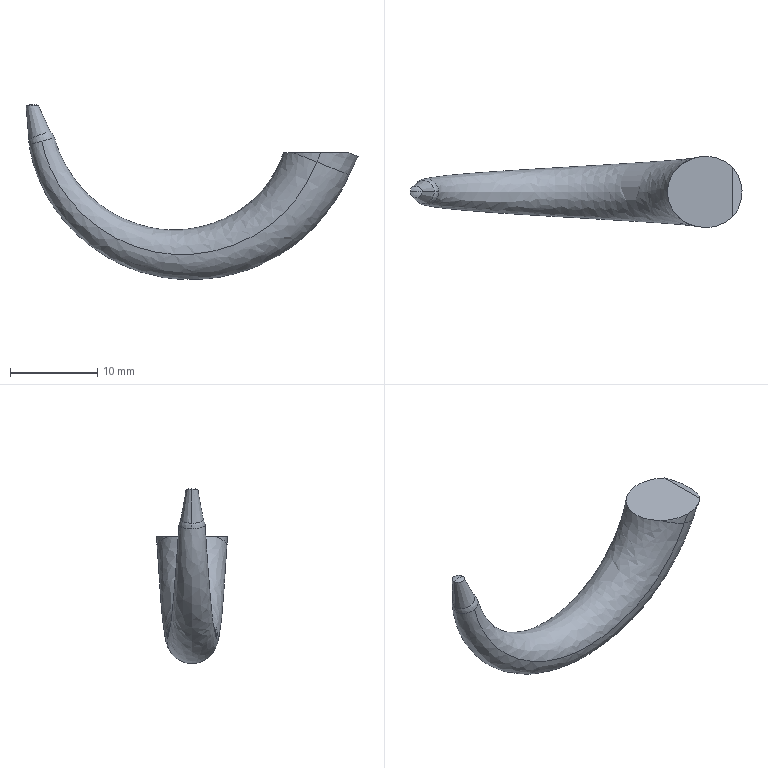Part | Creo | 1 solid | 13 faces | box 38.084 x 8.15 x 20.091 mm | volume 1170 mm3 | spline 5 | sphere 4 | plane 2 | cone 2
STEP:
#1=CARTESIAN_POINT('',(-144.079,122.31,36.852));
#2=VERTEX_POINT('',#1);
#3=CARTESIAN_POINT('',(-144.079,127.996,36.852));
#4=VERTEX_POINT('',#3);
#5=CARTESIAN_POINT('',(-144.079,122.31,36.852));
#6=DIRECTION('',(-0.000000028,1.,-0.000000063));
#7=VECTOR('',#6,5.687);
#8=LINE('',#5,#7);
#9=EDGE_CURVE('',#2,#4,#8,.T.);
#10=ORIENTED_EDGE('',*,*,#9,.F.);
#11=CARTESIAN_POINT('',(-147.308,121.079,36.852));
#12=VERTEX_POINT('',#11);
#13=CARTESIAN_POINT('',(-144.079,122.31,36.852));
#14=CARTESIAN_POINT('',(-144.243,122.153,36.852));
#15=CARTESIAN_POINT('',(-144.595,121.866,36.852));
#16=CARTESIAN_POINT('',(-145.204,121.513,36.852));
#17=CARTESIAN_POINT('',(-145.872,121.255,36.852));
#18=CARTESIAN_POINT('',(-146.584,121.102,36.852));
#19=CARTESIAN_POINT('',(-147.064,121.074,36.852));
#20=CARTESIAN_POINT('',(-147.308,121.079,36.852));
#21=B_SPLINE_CURVE_WITH_KNOTS('',3,(#13,#14,#15,#16,#17,#18,#19,#20),.UNSPECIFIED.,.F.,.F.,(4,1,1,1,1,4),(0.,0.2,0.4,0.6,0.8,1.),.UNSPECIFIED.);
#22=EDGE_CURVE('',#2,#12,#21,.T.);
#23=ORIENTED_EDGE('',*,*,#22,.T.);
#24=CARTESIAN_POINT('',(-150.452,122.415,36.852));
#25=VERTEX_POINT('',#24);
#26=CARTESIAN_POINT('',(-147.308,121.079,36.852));
#27=CARTESIAN_POINT('',(-147.55,121.084,36.852));
#28=CARTESIAN_POINT('',(-148.025,121.13,36.852));
#29=CARTESIAN_POINT('',(-148.724,121.309,36.852));
#30=CARTESIAN_POINT('',(-149.372,121.588,36.852));
#31=CARTESIAN_POINT('',(-149.957,121.957,36.852));
#32=CARTESIAN_POINT('',(-150.296,122.254,36.852));
#33=CARTESIAN_POINT('',(-150.451,122.414,36.852));
#34=B_SPLINE_CURVE_WITH_KNOTS('',3,(#26,#27,#28,#29,#30,#31,#32,#33),.UNSPECIFIED.,.F.,.F.,(4,1,1,1,1,4),(0.,0.2,0.4,0.6,0.8,1.),.UNSPECIFIED.);
#35=EDGE_CURVE('',#12,#25,#34,.T.);
#36=ORIENTED_EDGE('',*,*,#35,.T.);
#37=CARTESIAN_POINT('',(-150.452,127.891,36.852));
#38=VERTEX_POINT('',#37);
#39=CARTESIAN_POINT('',(-150.451,122.414,36.852));
#40=CARTESIAN_POINT('',(-150.618,122.585,36.852));
#41=CARTESIAN_POINT('',(-150.912,122.943,36.852));
#42=CARTESIAN_POINT('',(-151.252,123.538,36.852));
#43=CARTESIAN_POINT('',(-151.48,124.169,36.852));
#44=CARTESIAN_POINT('',(-151.596,124.824,36.852));
#45=CARTESIAN_POINT('',(-151.596,125.483,36.852));
#46=CARTESIAN_POINT('',(-151.48,126.137,36.852));
#47=CARTESIAN_POINT('',(-151.251,126.77,36.852));
#48=CARTESIAN_POINT('',(-150.91,127.364,36.852));
#49=CARTESIAN_POINT('',(-150.617,127.721,36.852));
#50=CARTESIAN_POINT('',(-150.452,127.892,36.852));
#51=B_SPLINE_CURVE_WITH_KNOTS('',3,(#39,#40,#41,#42,#43,#44,#45,#46,#47,#48,#49,#50),.UNSPECIFIED.,.F.,.F.,(4,1,1,1,1,1,1,1,1,4),(0.,0.1111,0.2222,0.3333,0.4444,0.5556,0.6667,0.7778,0.8889,1.),.UNSPECIFIED.);
#52=EDGE_CURVE('',#25,#38,#51,.T.);
#53=ORIENTED_EDGE('',*,*,#52,.T.);
#54=CARTESIAN_POINT('',(-147.308,129.227,36.852));
#55=VERTEX_POINT('',#54);
#56=CARTESIAN_POINT('',(-150.452,127.892,36.852));
#57=CARTESIAN_POINT('',(-150.296,128.052,36.852));
#58=CARTESIAN_POINT('',(-149.958,128.349,36.852));
#59=CARTESIAN_POINT('',(-149.373,128.717,36.852));
#60=CARTESIAN_POINT('',(-148.725,128.997,36.852));
#61=CARTESIAN_POINT('',(-148.029,129.175,36.852));
#62=CARTESIAN_POINT('',(-147.551,129.222,36.852));
#63=CARTESIAN_POINT('',(-147.308,129.227,36.852));
#64=B_SPLINE_CURVE_WITH_KNOTS('',3,(#56,#57,#58,#59,#60,#61,#62,#63),.UNSPECIFIED.,.F.,.F.,(4,1,1,1,1,4),(0.,0.2,0.4,0.6,0.8,1.),.UNSPECIFIED.);
#65=EDGE_CURVE('',#38,#55,#64,.T.);
#66=ORIENTED_EDGE('',*,*,#65,.T.);
#67=CARTESIAN_POINT('',(-144.079,127.996,36.852));
#68=CARTESIAN_POINT('',(-144.216,128.127,36.852));
#69=CARTESIAN_POINT('',(-144.506,128.369,36.852));
#70=CARTESIAN_POINT('',(-144.996,128.68,36.852));
#71=CARTESIAN_POINT('',(-145.532,128.928,36.852));
#72=CARTESIAN_POINT('',(-146.104,129.108,36.852));
#73=CARTESIAN_POINT('',(-146.7,129.213,36.852));
#74=CARTESIAN_POINT('',(-147.104,129.231,36.852));
#75=CARTESIAN_POINT('',(-147.308,129.227,36.852));
#76=B_SPLINE_CURVE_WITH_KNOTS('',3,(#67,#68,#69,#70,#71,#72,#73,#74,#75),.UNSPECIFIED.,.F.,.F.,(4,1,1,1,1,1,4),(0.,0.1667,0.3333,0.5,0.6667,0.8333,1.),.UNSPECIFIED.);
#77=EDGE_CURVE('',#4,#55,#76,.T.);
#78=ORIENTED_EDGE('',*,*,#77,.F.);
#79=EDGE_LOOP('',(#10,#23,#36,#53,#66,#78));
#80=FACE_OUTER_BOUND('',#79,.F.);
#81=CARTESIAN_POINT('',(-151.801,125.153,36.852));
#82=DIRECTION('',(0.,0.,1.));
#83=DIRECTION('',(1.,0.,0.));
#84=AXIS2_PLACEMENT_3D('',#81,#82,#83);
#85=PLANE('',#84);
#86=ADVANCED_FACE('',(#80),#85,.T.);
#87=CARTESIAN_POINT('',(-144.079,127.996,36.852));
#88=CARTESIAN_POINT('',(-143.93,127.825,36.793));
#89=CARTESIAN_POINT('',(-143.662,127.463,36.687));
#90=CARTESIAN_POINT('',(-143.348,126.85,36.562));
#91=CARTESIAN_POINT('',(-143.134,126.191,36.477));
#92=CARTESIAN_POINT('',(-143.026,125.502,36.434));
#93=CARTESIAN_POINT('',(-143.026,124.804,36.434));
#94=CARTESIAN_POINT('',(-143.134,124.115,36.477));
#95=CARTESIAN_POINT('',(-143.348,123.456,36.562));
#96=CARTESIAN_POINT('',(-143.662,122.843,36.687));
#97=CARTESIAN_POINT('',(-143.93,122.481,36.793));
#98=CARTESIAN_POINT('',(-144.079,122.31,36.852));
#99=B_SPLINE_CURVE_WITH_KNOTS('',3,(#87,#88,#89,#90,#91,#92,#93,#94,#95,#96,#97,#98),.UNSPECIFIED.,.F.,.F.,(4,1,1,1,1,1,1,1,1,4),(0.,0.1111,0.2222,0.3333,0.4444,0.5556,0.6667,0.7778,0.8889,1.),.UNSPECIFIED.);
#100=EDGE_CURVE('',#4,#2,#99,.T.);
#101=ORIENTED_EDGE('',*,*,#100,.T.);
#102=ORIENTED_EDGE('',*,*,#9,.T.);
#103=EDGE_LOOP('',(#101,#102));
#104=FACE_OUTER_BOUND('',#103,.F.);
#105=CARTESIAN_POINT('',(-145.561,129.153,37.44));
#106=DIRECTION('',(0.3687,0.,0.9295));
#107=DIRECTION('',(-0.9295,0.,0.3687));
#108=AXIS2_PLACEMENT_3D('',#105,#106,#107);
#109=PLANE('',#108);
#110=ADVANCED_FACE('',(#104),#109,.T.);
#111=ORIENTED_EDGE('',*,*,#22,.F.);
#112=ORIENTED_EDGE('',*,*,#100,.F.);
#113=ORIENTED_EDGE('',*,*,#77,.T.);
#114=CARTESIAN_POINT('',(-147.742,129.153,35.777));
#115=VERTEX_POINT('',#114);
#116=CARTESIAN_POINT('',(-147.308,129.227,36.852));
#117=DIRECTION('',(-0.3736,-0.06365,-0.9254));
#118=VECTOR('',#117,1.162);
#119=LINE('',#116,#118);
#120=EDGE_CURVE('',#55,#115,#119,.T.);
#121=ORIENTED_EDGE('',*,*,#120,.T.);
#122=CARTESIAN_POINT('',(-147.742,121.153,35.777));
#123=VERTEX_POINT('',#122);
#124=CARTESIAN_POINT('',(-147.742,125.153,35.777));
#125=DIRECTION('',(0.3687,0.,0.9295));
#126=DIRECTION('',(0.,-1.,0.));
#127=AXIS2_PLACEMENT_3D('',#124,#125,#126);
#128=CIRCLE('',#127,4.);
#129=EDGE_CURVE('',#123,#115,#128,.T.);
#130=ORIENTED_EDGE('',*,*,#129,.F.);
#131=CARTESIAN_POINT('',(-147.308,121.079,36.852));
#132=DIRECTION('',(-0.3735,0.06365,-0.9254));
#133=VECTOR('',#132,1.162);
#134=LINE('',#131,#133);
#135=EDGE_CURVE('',#12,#123,#134,.T.);
#136=ORIENTED_EDGE('',*,*,#135,.F.);
#137=EDGE_LOOP('',(#111,#112,#113,#121,#130,#136));
#138=FACE_OUTER_BOUND('',#137,.F.);
#139=CARTESIAN_POINT('',(-147.195,121.027,37.769));
#140=CARTESIAN_POINT('',(-147.462,121.073,37.12));
#141=CARTESIAN_POINT('',(-147.728,121.119,36.471));
#142=CARTESIAN_POINT('',(-147.995,121.164,35.821));
#143=CARTESIAN_POINT('',(-147.117,121.023,37.748));
#144=CARTESIAN_POINT('',(-147.384,121.068,37.095));
#145=CARTESIAN_POINT('',(-147.651,121.114,36.443));
#146=CARTESIAN_POINT('',(-147.918,121.159,35.79));
#147=CARTESIAN_POINT('',(-147.04,121.02,37.727));
#148=CARTESIAN_POINT('',(-147.307,121.066,37.071));
#149=CARTESIAN_POINT('',(-147.573,121.111,36.415));
#150=CARTESIAN_POINT('',(-147.84,121.156,35.759));
#151=CARTESIAN_POINT('',(-146.722,121.02,37.64));
#152=CARTESIAN_POINT('',(-146.987,121.066,36.97));
#153=CARTESIAN_POINT('',(-147.253,121.111,36.3));
#154=CARTESIAN_POINT('',(-147.518,121.156,35.631));
#155=CARTESIAN_POINT('',(-146.24,121.064,37.507));
#156=CARTESIAN_POINT('',(-146.504,121.112,36.817));
#157=CARTESIAN_POINT('',(-146.768,121.16,36.126));
#158=CARTESIAN_POINT('',(-147.031,121.208,35.436));
#159=CARTESIAN_POINT('',(-145.231,121.354,37.231));
#160=CARTESIAN_POINT('',(-145.519,121.407,36.508));
#161=CARTESIAN_POINT('',(-145.808,121.461,35.785));
#162=CARTESIAN_POINT('',(-146.097,121.514,35.062));
#163=CARTESIAN_POINT('',(-144.042,122.144,36.904));
#164=CARTESIAN_POINT('',(-144.385,122.18,36.153));
#165=CARTESIAN_POINT('',(-144.727,122.217,35.402));
#166=CARTESIAN_POINT('',(-145.07,122.254,34.651));
#167=CARTESIAN_POINT('',(-143.276,123.368,36.694));
#168=CARTESIAN_POINT('',(-143.645,123.366,35.921));
#169=CARTESIAN_POINT('',(-144.014,123.363,35.149));
#170=CARTESIAN_POINT('',(-144.383,123.36,34.376));
#171=CARTESIAN_POINT('',(-142.994,124.408,36.617));
#172=CARTESIAN_POINT('',(-143.362,124.394,35.832));
#173=CARTESIAN_POINT('',(-143.731,124.38,35.047));
#174=CARTESIAN_POINT('',(-144.099,124.367,34.263));
#175=CARTESIAN_POINT('',(-142.931,125.153,36.6));
#176=CARTESIAN_POINT('',(-143.296,125.153,35.811));
#177=CARTESIAN_POINT('',(-143.661,125.153,35.022));
#178=CARTESIAN_POINT('',(-144.027,125.153,34.234));
#179=CARTESIAN_POINT('',(-142.994,125.898,36.617));
#180=CARTESIAN_POINT('',(-143.362,125.912,35.832));
#181=CARTESIAN_POINT('',(-143.731,125.926,35.047));
#182=CARTESIAN_POINT('',(-144.099,125.939,34.263));
#183=CARTESIAN_POINT('',(-143.276,126.938,36.694));
#184=CARTESIAN_POINT('',(-143.645,126.94,35.921));
#185=CARTESIAN_POINT('',(-144.014,126.943,35.149));
#186=CARTESIAN_POINT('',(-144.383,126.946,34.376));
#187=CARTESIAN_POINT('',(-144.042,128.162,36.904));
#188=CARTESIAN_POINT('',(-144.385,128.126,36.153));
#189=CARTESIAN_POINT('',(-144.727,128.089,35.402));
#190=CARTESIAN_POINT('',(-145.07,128.052,34.651));
#191=CARTESIAN_POINT('',(-145.231,128.952,37.231));
#192=CARTESIAN_POINT('',(-145.519,128.899,36.508));
#193=CARTESIAN_POINT('',(-145.808,128.845,35.785));
#194=CARTESIAN_POINT('',(-146.097,128.792,35.062));
#195=CARTESIAN_POINT('',(-146.24,129.242,37.507));
#196=CARTESIAN_POINT('',(-146.504,129.194,36.817));
#197=CARTESIAN_POINT('',(-146.768,129.146,36.126));
#198=CARTESIAN_POINT('',(-147.031,129.098,35.436));
#199=CARTESIAN_POINT('',(-146.799,129.293,37.661));
#200=CARTESIAN_POINT('',(-147.065,129.248,36.994));
#201=CARTESIAN_POINT('',(-147.33,129.203,36.328));
#202=CARTESIAN_POINT('',(-147.596,129.158,35.662));
#203=CARTESIAN_POINT('',(-147.117,129.283,37.748));
#204=CARTESIAN_POINT('',(-147.384,129.238,37.095));
#205=CARTESIAN_POINT('',(-147.651,129.192,36.443));
#206=CARTESIAN_POINT('',(-147.917,129.147,35.79));
#207=CARTESIAN_POINT('',(-147.195,129.279,37.769));
#208=CARTESIAN_POINT('',(-147.461,129.233,37.12));
#209=CARTESIAN_POINT('',(-147.728,129.188,36.47));
#210=CARTESIAN_POINT('',(-147.995,129.142,35.821));
#211=B_SPLINE_SURFACE_WITH_KNOTS('',3,3,((#139,#140,#141,#142),(#143,#144,#145,#146),(#147,#148,#149,#150),(#151,#152,#153,#154),(#155,#156,#157,#158),(#159,#160,#161,#162),(#163,#164,#165,#166),(#167,#168,#169,#170),(#171,#172,#173,#174),(#175,#176,#177,#178),(#179,#180,#181,#182),(#183,#184,#185,#186),(#187,#188,#189,#190),(#191,#192,#193,#194),(#195,#196,#197,#198),(#199,#200,#201,#202),(#203,#204,#205,#206),(#207,#208,#209,#210)),.UNSPECIFIED.,.F.,.F.,.F.,(4,1,1,1,1,1,1,1,1,1,1,1,1,1,1,4),(4,4),(-0.02,0.,0.00001571,0.06251,0.125,0.25,0.375,0.4375,0.5,0.5625,0.625,0.75,0.875,0.9375,1.,1.02),(-0.026,1.026),.UNSPECIFIED.);
#212=ADVANCED_FACE('',(#138),#211,.F.);
#213=ORIENTED_EDGE('',*,*,#35,.F.);
#214=ORIENTED_EDGE('',*,*,#135,.T.);
#215=CARTESIAN_POINT('',(-147.742,125.153,35.777));
#216=DIRECTION('',(0.3688,0.,0.9295));
#217=DIRECTION('',(-0.6777,-0.6845,0.2688));
#218=AXIS2_PLACEMENT_3D('',#215,#216,#217);
#219=CIRCLE('',#218,4.);
#220=EDGE_CURVE('',#25,#123,#219,.T.);
#221=ORIENTED_EDGE('',*,*,#220,.F.);
#222=EDGE_LOOP('',(#213,#214,#221));
#223=FACE_OUTER_BOUND('',#222,.F.);
#224=CARTESIAN_POINT('',(-147.064,129.224,36.828));
#225=CARTESIAN_POINT('',(-147.219,129.196,36.43));
#226=CARTESIAN_POINT('',(-147.373,129.169,36.032));
#227=CARTESIAN_POINT('',(-147.528,129.142,35.634));
#228=CARTESIAN_POINT('',(-147.139,129.228,36.852));
#229=CARTESIAN_POINT('',(-147.294,129.201,36.457));
#230=CARTESIAN_POINT('',(-147.45,129.174,36.061));
#231=CARTESIAN_POINT('',(-147.606,129.147,35.665));
#232=CARTESIAN_POINT('',(-147.447,129.237,36.952));
#233=CARTESIAN_POINT('',(-147.607,129.211,36.566));
#234=CARTESIAN_POINT('',(-147.767,129.184,36.18));
#235=CARTESIAN_POINT('',(-147.927,129.158,35.794));
#236=CARTESIAN_POINT('',(-147.988,129.188,37.126));
#237=CARTESIAN_POINT('',(-148.156,129.158,36.758));
#238=CARTESIAN_POINT('',(-148.325,129.128,36.389));
#239=CARTESIAN_POINT('',(-148.493,129.098,36.02));
#240=CARTESIAN_POINT('',(-148.966,128.902,37.443));
#241=CARTESIAN_POINT('',(-149.12,128.865,37.093));
#242=CARTESIAN_POINT('',(-149.274,128.828,36.743));
#243=CARTESIAN_POINT('',(-149.427,128.792,36.394));
#244=CARTESIAN_POINT('',(-150.12,128.122,37.816));
#245=CARTESIAN_POINT('',(-150.231,128.099,37.479));
#246=CARTESIAN_POINT('',(-150.342,128.076,37.142));
#247=CARTESIAN_POINT('',(-150.453,128.052,36.805));
#248=CARTESIAN_POINT('',(-150.864,126.913,38.056));
#249=CARTESIAN_POINT('',(-150.956,126.924,37.73));
#250=CARTESIAN_POINT('',(-151.048,126.935,37.405));
#251=CARTESIAN_POINT('',(-151.14,126.947,37.079));
#252=CARTESIAN_POINT('',(-151.137,125.887,38.144));
#253=CARTESIAN_POINT('',(-151.232,125.905,37.827));
#254=CARTESIAN_POINT('',(-151.328,125.923,37.51));
#255=CARTESIAN_POINT('',(-151.424,125.941,37.193));
#256=CARTESIAN_POINT('',(-151.197,125.153,38.164));
#257=CARTESIAN_POINT('',(-151.297,125.153,37.85));
#258=CARTESIAN_POINT('',(-151.397,125.153,37.536));
#259=CARTESIAN_POINT('',(-151.496,125.153,37.222));
#260=CARTESIAN_POINT('',(-151.137,124.419,38.144));
#261=CARTESIAN_POINT('',(-151.232,124.401,37.827));
#262=CARTESIAN_POINT('',(-151.328,124.383,37.51));
#263=CARTESIAN_POINT('',(-151.424,124.365,37.193));
#264=CARTESIAN_POINT('',(-150.864,123.393,38.056));
#265=CARTESIAN_POINT('',(-150.956,123.382,37.73));
#266=CARTESIAN_POINT('',(-151.048,123.371,37.405));
#267=CARTESIAN_POINT('',(-151.14,123.359,37.079));
#268=CARTESIAN_POINT('',(-150.12,122.184,37.816));
#269=CARTESIAN_POINT('',(-150.231,122.207,37.479));
#270=CARTESIAN_POINT('',(-150.342,122.23,37.142));
#271=CARTESIAN_POINT('',(-150.453,122.254,36.805));
#272=CARTESIAN_POINT('',(-148.966,121.404,37.443));
#273=CARTESIAN_POINT('',(-149.12,121.441,37.093));
#274=CARTESIAN_POINT('',(-149.274,121.478,36.743));
#275=CARTESIAN_POINT('',(-149.427,121.514,36.394));
#276=CARTESIAN_POINT('',(-147.988,121.118,37.126));
#277=CARTESIAN_POINT('',(-148.156,121.148,36.758));
#278=CARTESIAN_POINT('',(-148.325,121.178,36.389));
#279=CARTESIAN_POINT('',(-148.493,121.208,36.02));
#280=CARTESIAN_POINT('',(-147.447,121.069,36.952));
#281=CARTESIAN_POINT('',(-147.607,121.095,36.566));
#282=CARTESIAN_POINT('',(-147.767,121.122,36.18));
#283=CARTESIAN_POINT('',(-147.927,121.148,35.794));
#284=CARTESIAN_POINT('',(-147.139,121.078,36.852));
#285=CARTESIAN_POINT('',(-147.294,121.105,36.457));
#286=CARTESIAN_POINT('',(-147.45,121.132,36.061));
#287=CARTESIAN_POINT('',(-147.606,121.159,35.665));
#288=CARTESIAN_POINT('',(-147.064,121.082,36.828));
#289=CARTESIAN_POINT('',(-147.219,121.11,36.43));
#290=CARTESIAN_POINT('',(-147.373,121.137,36.032));
#291=CARTESIAN_POINT('',(-147.528,121.164,35.634));
#292=B_SPLINE_SURFACE_WITH_KNOTS('',3,3,((#224,#225,#226,#227),(#228,#229,#230,#231),(#232,#233,#234,#235),(#236,#237,#238,#239),(#240,#241,#242,#243),(#244,#245,#246,#247),(#248,#249,#250,#251),(#252,#253,#254,#255),(#256,#257,#258,#259),(#260,#261,#262,#263),(#264,#265,#266,#267),(#268,#269,#270,#271),(#272,#273,#274,#275),(#276,#277,#278,#279),(#280,#281,#282,#283),(#284,#285,#286,#287),(#288,#289,#290,#291)),.UNSPECIFIED.,.F.,.F.,.F.,(4,1,1,1,1,1,1,1,1,1,1,1,1,1,4),(4,4),(-0.02,0.,0.0625,0.125,0.25,0.375,0.4375,0.5,0.5625,0.625,0.75,0.875,0.9375,1.,1.02),(-0.04546,1.045),.UNSPECIFIED.);
#293=ADVANCED_FACE('',(#223),#292,.F.);
#294=ORIENTED_EDGE('',*,*,#65,.F.);
#295=CARTESIAN_POINT('',(-147.742,125.153,35.777));
#296=DIRECTION('',(0.3688,0.,0.9295));
#297=DIRECTION('',(0.000000184,1.,-0.000000073));
#298=AXIS2_PLACEMENT_3D('',#295,#296,#297);
#299=CIRCLE('',#298,4.);
#300=EDGE_CURVE('',#115,#38,#299,.T.);
#301=ORIENTED_EDGE('',*,*,#300,.F.);
#302=ORIENTED_EDGE('',*,*,#120,.F.);
#303=EDGE_LOOP('',(#294,#301,#302));
#304=FACE_OUTER_BOUND('',#303,.F.);
#305=CARTESIAN_POINT('',(-147.064,129.224,36.828));
#306=CARTESIAN_POINT('',(-147.219,129.196,36.43));
#307=CARTESIAN_POINT('',(-147.373,129.169,36.032));
#308=CARTESIAN_POINT('',(-147.528,129.142,35.634));
#309=CARTESIAN_POINT('',(-147.139,129.228,36.852));
#310=CARTESIAN_POINT('',(-147.294,129.201,36.457));
#311=CARTESIAN_POINT('',(-147.45,129.174,36.061));
#312=CARTESIAN_POINT('',(-147.606,129.147,35.665));
#313=CARTESIAN_POINT('',(-147.447,129.237,36.952));
#314=CARTESIAN_POINT('',(-147.607,129.211,36.566));
#315=CARTESIAN_POINT('',(-147.767,129.184,36.18));
#316=CARTESIAN_POINT('',(-147.927,129.158,35.794));
#317=CARTESIAN_POINT('',(-147.988,129.188,37.126));
#318=CARTESIAN_POINT('',(-148.156,129.158,36.758));
#319=CARTESIAN_POINT('',(-148.325,129.128,36.389));
#320=CARTESIAN_POINT('',(-148.493,129.098,36.02));
#321=CARTESIAN_POINT('',(-148.966,128.902,37.443));
#322=CARTESIAN_POINT('',(-149.12,128.865,37.093));
#323=CARTESIAN_POINT('',(-149.274,128.828,36.743));
#324=CARTESIAN_POINT('',(-149.427,128.792,36.394));
#325=CARTESIAN_POINT('',(-150.12,128.122,37.816));
#326=CARTESIAN_POINT('',(-150.231,128.099,37.479));
#327=CARTESIAN_POINT('',(-150.342,128.076,37.142));
#328=CARTESIAN_POINT('',(-150.453,128.052,36.805));
#329=CARTESIAN_POINT('',(-150.864,126.913,38.056));
#330=CARTESIAN_POINT('',(-150.956,126.924,37.73));
#331=CARTESIAN_POINT('',(-151.048,126.935,37.405));
#332=CARTESIAN_POINT('',(-151.14,126.947,37.079));
#333=CARTESIAN_POINT('',(-151.137,125.887,38.144));
#334=CARTESIAN_POINT('',(-151.232,125.905,37.827));
#335=CARTESIAN_POINT('',(-151.328,125.923,37.51));
#336=CARTESIAN_POINT('',(-151.424,125.941,37.193));
#337=CARTESIAN_POINT('',(-151.197,125.153,38.164));
#338=CARTESIAN_POINT('',(-151.297,125.153,37.85));
#339=CARTESIAN_POINT('',(-151.397,125.153,37.536));
#340=CARTESIAN_POINT('',(-151.496,125.153,37.222));
#341=CARTESIAN_POINT('',(-151.137,124.419,38.144));
#342=CARTESIAN_POINT('',(-151.232,124.401,37.827));
#343=CARTESIAN_POINT('',(-151.328,124.383,37.51));
#344=CARTESIAN_POINT('',(-151.424,124.365,37.193));
#345=CARTESIAN_POINT('',(-150.864,123.393,38.056));
#346=CARTESIAN_POINT('',(-150.956,123.382,37.73));
#347=CARTESIAN_POINT('',(-151.048,123.371,37.405));
#348=CARTESIAN_POINT('',(-151.14,123.359,37.079));
#349=CARTESIAN_POINT('',(-150.12,122.184,37.816));
#350=CARTESIAN_POINT('',(-150.231,122.207,37.479));
#351=CARTESIAN_POINT('',(-150.342,122.23,37.142));
#352=CARTESIAN_POINT('',(-150.453,122.254,36.805));
#353=CARTESIAN_POINT('',(-148.966,121.404,37.443));
#354=CARTESIAN_POINT('',(-149.12,121.441,37.093));
#355=CARTESIAN_POINT('',(-149.274,121.478,36.743));
#356=CARTESIAN_POINT('',(-149.427,121.514,36.394));
#357=CARTESIAN_POINT('',(-147.988,121.118,37.126));
#358=CARTESIAN_POINT('',(-148.156,121.148,36.758));
#359=CARTESIAN_POINT('',(-148.325,121.178,36.389));
#360=CARTESIAN_POINT('',(-148.493,121.208,36.02));
#361=CARTESIAN_POINT('',(-147.447,121.069,36.952));
#362=CARTESIAN_POINT('',(-147.607,121.095,36.566));
#363=CARTESIAN_POINT('',(-147.767,121.122,36.18));
#364=CARTESIAN_POINT('',(-147.927,121.148,35.794));
#365=CARTESIAN_POINT('',(-147.139,121.078,36.852));
#366=CARTESIAN_POINT('',(-147.294,121.105,36.457));
#367=CARTESIAN_POINT('',(-147.45,121.132,36.061));
#368=CARTESIAN_POINT('',(-147.606,121.159,35.665));
#369=CARTESIAN_POINT('',(-147.064,121.082,36.828));
#370=CARTESIAN_POINT('',(-147.219,121.11,36.43));
#371=CARTESIAN_POINT('',(-147.373,121.137,36.032));
#372=CARTESIAN_POINT('',(-147.528,121.164,35.634));
#373=B_SPLINE_SURFACE_WITH_KNOTS('',3,3,((#305,#306,#307,#308),(#309,#310,#311,#312),(#313,#314,#315,#316),(#317,#318,#319,#320),(#321,#322,#323,#324),(#325,#326,#327,#328),(#329,#330,#331,#332),(#333,#334,#335,#336),(#337,#338,#339,#340),(#341,#342,#343,#344),(#345,#346,#347,#348),(#349,#350,#351,#352),(#353,#354,#355,#356),(#357,#358,#359,#360),(#361,#362,#363,#364),(#365,#366,#367,#368),(#369,#370,#371,#372)),.UNSPECIFIED.,.F.,.F.,.F.,(4,1,1,1,1,1,1,1,1,1,1,1,1,1,4),(4,4),(-0.02,0.,0.0625,0.125,0.25,0.375,0.4375,0.5,0.5625,0.625,0.75,0.875,0.9375,1.,1.02),(-0.04546,1.045),.UNSPECIFIED.);
#374=ADVANCED_FACE('',(#304),#373,.F.);
#375=ORIENTED_EDGE('',*,*,#52,.F.);
#376=ORIENTED_EDGE('',*,*,#220,.T.);
#377=CARTESIAN_POINT('',(-179.3,123.653,38.166));
#378=VERTEX_POINT('',#377);
#379=CARTESIAN_POINT('',(-147.742,121.153,35.777));
#380=CARTESIAN_POINT('',(-148.818,121.336,33.111));
#381=CARTESIAN_POINT('',(-153.097,121.702,26.957));
#382=CARTESIAN_POINT('',(-167.8,122.536,22.647));
#383=CARTESIAN_POINT('',(-177.88,123.191,31.227));
#384=B_SPLINE_CURVE_WITH_KNOTS('',3,(#379,#380,#381,#382,#383,#377),.UNSPECIFIED.,.F.,.F.,(4,1,1,4),(0.,0.1926,0.52,1.),.UNSPECIFIED.);
#385=EDGE_CURVE('',#123,#378,#384,.T.);
#386=ORIENTED_EDGE('',*,*,#385,.T.);
#387=CARTESIAN_POINT('',(-177.856,125.153,38.573));
#388=VERTEX_POINT('',#387);
#389=CARTESIAN_POINT('',(-177.856,125.153,38.573));
#390=CARTESIAN_POINT('',(-177.856,125.063,38.573));
#391=CARTESIAN_POINT('',(-177.871,124.882,38.569));
#392=CARTESIAN_POINT('',(-177.948,124.599,38.547));
#393=CARTESIAN_POINT('',(-178.082,124.327,38.509));
#394=CARTESIAN_POINT('',(-178.334,124.003,38.438));
#395=CARTESIAN_POINT('',(-178.676,123.774,38.342));
#396=CARTESIAN_POINT('',(-178.993,123.682,38.252));
#397=CARTESIAN_POINT('',(-179.171,123.657,38.202));
#398=CARTESIAN_POINT('',(-179.257,123.653,38.178));
#399=CARTESIAN_POINT('',(-179.3,123.653,38.166));
#400=B_SPLINE_CURVE_WITH_KNOTS('',3,(#389,#390,#391,#392,#393,#394,#395,#396,#397,#398,#399),.UNSPECIFIED.,.F.,.F.,(4,1,1,1,1,1,1,1,4),(0.,0.125,0.25,0.375,0.5,0.75,0.875,0.9375,1.),.UNSPECIFIED.);
#401=EDGE_CURVE('',#388,#378,#400,.T.);
#402=ORIENTED_EDGE('',*,*,#401,.F.);
#403=CARTESIAN_POINT('',(-179.3,126.653,38.166));
#404=VERTEX_POINT('',#403);
#405=CARTESIAN_POINT('',(-179.3,126.653,38.166));
#406=CARTESIAN_POINT('',(-179.257,126.653,38.178));
#407=CARTESIAN_POINT('',(-179.171,126.649,38.202));
#408=CARTESIAN_POINT('',(-178.993,126.624,38.252));
#409=CARTESIAN_POINT('',(-178.676,126.532,38.342));
#410=CARTESIAN_POINT('',(-178.334,126.303,38.438));
#411=CARTESIAN_POINT('',(-178.082,125.979,38.509));
#412=CARTESIAN_POINT('',(-177.948,125.707,38.547));
#413=CARTESIAN_POINT('',(-177.871,125.424,38.569));
#414=CARTESIAN_POINT('',(-177.856,125.243,38.573));
#415=CARTESIAN_POINT('',(-177.856,125.153,38.573));
#416=B_SPLINE_CURVE_WITH_KNOTS('',3,(#405,#406,#407,#408,#409,#410,#411,#412,#413,#414,#415),.UNSPECIFIED.,.F.,.F.,(4,1,1,1,1,1,1,1,4),(0.,0.0625,0.125,0.25,0.5,0.625,0.75,0.875,1.),.UNSPECIFIED.);
#417=EDGE_CURVE('',#404,#388,#416,.T.);
#418=ORIENTED_EDGE('',*,*,#417,.F.);
#419=CARTESIAN_POINT('',(-147.742,129.153,35.777));
#420=CARTESIAN_POINT('',(-148.818,128.97,33.111));
#421=CARTESIAN_POINT('',(-153.097,128.604,26.957));
#422=CARTESIAN_POINT('',(-167.8,127.77,22.647));
#423=CARTESIAN_POINT('',(-177.88,127.115,31.227));
#424=B_SPLINE_CURVE_WITH_KNOTS('',3,(#419,#420,#421,#422,#423,#403),.UNSPECIFIED.,.F.,.F.,(4,1,1,4),(0.,0.1926,0.52,1.),.UNSPECIFIED.);
#425=EDGE_CURVE('',#115,#404,#424,.T.);
#426=ORIENTED_EDGE('',*,*,#425,.F.);
#427=ORIENTED_EDGE('',*,*,#300,.T.);
#428=EDGE_LOOP('',(#375,#376,#386,#402,#418,#426,#427));
#429=FACE_OUTER_BOUND('',#428,.F.);
#430=CARTESIAN_POINT('',(-147.378,129.172,36.072));
#431=CARTESIAN_POINT('',(-148.479,128.976,33.212));
#432=CARTESIAN_POINT('',(-152.845,128.605,26.82));
#433=CARTESIAN_POINT('',(-167.979,127.759,22.434));
#434=CARTESIAN_POINT('',(-178.203,127.098,31.352));
#435=CARTESIAN_POINT('',(-179.456,126.625,38.533));
#436=CARTESIAN_POINT('',(-147.451,129.177,36.099));
#437=CARTESIAN_POINT('',(-148.544,128.98,33.25));
#438=CARTESIAN_POINT('',(-152.885,128.609,26.879));
#439=CARTESIAN_POINT('',(-167.962,127.762,22.492));
#440=CARTESIAN_POINT('',(-178.169,127.1,31.374));
#441=CARTESIAN_POINT('',(-179.428,126.626,38.54));
#442=CARTESIAN_POINT('',(-147.635,129.182,36.168));
#443=CARTESIAN_POINT('',(-148.707,128.985,33.346));
#444=CARTESIAN_POINT('',(-152.988,128.614,27.028));
#445=CARTESIAN_POINT('',(-167.921,127.765,22.641));
#446=CARTESIAN_POINT('',(-178.083,127.102,31.43));
#447=CARTESIAN_POINT('',(-179.358,126.628,38.558));
#448=CARTESIAN_POINT('',(-147.932,129.169,36.278));
#449=CARTESIAN_POINT('',(-148.971,128.972,33.499));
#450=CARTESIAN_POINT('',(-153.153,128.602,27.269));
#451=CARTESIAN_POINT('',(-167.855,127.756,22.881));
#452=CARTESIAN_POINT('',(-177.944,127.096,31.521));
#453=CARTESIAN_POINT('',(-179.246,126.623,38.586));
#454=CARTESIAN_POINT('',(-148.397,129.101,36.451));
#455=CARTESIAN_POINT('',(-149.385,128.908,33.74));
#456=CARTESIAN_POINT('',(-153.412,128.544,27.646));
#457=CARTESIAN_POINT('',(-167.752,127.713,23.257));
#458=CARTESIAN_POINT('',(-177.727,127.063,31.664));
#459=CARTESIAN_POINT('',(-179.071,126.599,38.631));
#460=CARTESIAN_POINT('',(-149.225,128.853,36.758));
#461=CARTESIAN_POINT('',(-150.121,128.672,34.169));
#462=CARTESIAN_POINT('',(-153.873,128.331,28.316));
#463=CARTESIAN_POINT('',(-167.568,127.552,23.925));
#464=CARTESIAN_POINT('',(-177.339,126.943,31.918));
#465=CARTESIAN_POINT('',(-178.758,126.508,38.711));
#466=CARTESIAN_POINT('',(-150.118,128.239,37.09));
#467=CARTESIAN_POINT('',(-150.915,128.088,34.632));
#468=CARTESIAN_POINT('',(-154.371,127.803,29.04));
#469=CARTESIAN_POINT('',(-167.369,127.153,24.647));
#470=CARTESIAN_POINT('',(-176.922,126.646,32.192));
#471=CARTESIAN_POINT('',(-178.42,126.283,38.797));
#472=CARTESIAN_POINT('',(-150.778,127.369,37.335));
#473=CARTESIAN_POINT('',(-151.501,127.26,34.974));
#474=CARTESIAN_POINT('',(-154.738,127.056,29.575));
#475=CARTESIAN_POINT('',(-167.222,126.59,25.179));
#476=CARTESIAN_POINT('',(-176.613,126.225,32.395));
#477=CARTESIAN_POINT('',(-178.171,125.964,38.86));
#478=CARTESIAN_POINT('',(-151.129,126.64,37.465));
#479=CARTESIAN_POINT('',(-151.814,126.568,35.156));
#480=CARTESIAN_POINT('',(-154.934,126.43,29.859));
#481=CARTESIAN_POINT('',(-167.144,126.117,25.463));
#482=CARTESIAN_POINT('',(-176.449,125.872,32.503));
#483=CARTESIAN_POINT('',(-178.038,125.698,38.894));
#484=CARTESIAN_POINT('',(-151.329,125.88,37.54));
#485=CARTESIAN_POINT('',(-151.992,125.845,35.26));
#486=CARTESIAN_POINT('',(-155.046,125.778,30.022));
#487=CARTESIAN_POINT('',(-167.099,125.624,25.625));
#488=CARTESIAN_POINT('',(-176.355,125.505,32.564));
#489=CARTESIAN_POINT('',(-177.963,125.419,38.913));
#490=CARTESIAN_POINT('',(-151.389,125.153,37.562));
#491=CARTESIAN_POINT('',(-152.044,125.153,35.291));
#492=CARTESIAN_POINT('',(-155.079,125.153,30.07));
#493=CARTESIAN_POINT('',(-167.086,125.153,25.673));
#494=CARTESIAN_POINT('',(-176.327,125.153,32.582));
#495=CARTESIAN_POINT('',(-177.94,125.153,38.919));
#496=CARTESIAN_POINT('',(-151.329,124.426,37.54));
#497=CARTESIAN_POINT('',(-151.992,124.461,35.26));
#498=CARTESIAN_POINT('',(-155.046,124.528,30.022));
#499=CARTESIAN_POINT('',(-167.099,124.682,25.625));
#500=CARTESIAN_POINT('',(-176.355,124.801,32.564));
#501=CARTESIAN_POINT('',(-177.963,124.887,38.913));
#502=CARTESIAN_POINT('',(-151.129,123.666,37.465));
#503=CARTESIAN_POINT('',(-151.814,123.738,35.156));
#504=CARTESIAN_POINT('',(-154.934,123.876,29.859));
#505=CARTESIAN_POINT('',(-167.144,124.189,25.463));
#506=CARTESIAN_POINT('',(-176.449,124.434,32.503));
#507=CARTESIAN_POINT('',(-178.038,124.608,38.894));
#508=CARTESIAN_POINT('',(-150.778,122.937,37.335));
#509=CARTESIAN_POINT('',(-151.501,123.046,34.974));
#510=CARTESIAN_POINT('',(-154.738,123.25,29.575));
#511=CARTESIAN_POINT('',(-167.222,123.716,25.179));
#512=CARTESIAN_POINT('',(-176.613,124.081,32.395));
#513=CARTESIAN_POINT('',(-178.171,124.342,38.86));
#514=CARTESIAN_POINT('',(-150.118,122.067,37.09));
#515=CARTESIAN_POINT('',(-150.915,122.218,34.632));
#516=CARTESIAN_POINT('',(-154.371,122.503,29.04));
#517=CARTESIAN_POINT('',(-167.369,123.153,24.647));
#518=CARTESIAN_POINT('',(-176.922,123.66,32.192));
#519=CARTESIAN_POINT('',(-178.42,124.023,38.797));
#520=CARTESIAN_POINT('',(-149.225,121.453,36.758));
#521=CARTESIAN_POINT('',(-150.121,121.634,34.169));
#522=CARTESIAN_POINT('',(-153.873,121.975,28.316));
#523=CARTESIAN_POINT('',(-167.568,122.754,23.925));
#524=CARTESIAN_POINT('',(-177.339,123.363,31.918));
#525=CARTESIAN_POINT('',(-178.758,123.798,38.711));
#526=CARTESIAN_POINT('',(-148.397,121.205,36.451));
#527=CARTESIAN_POINT('',(-149.385,121.398,33.74));
#528=CARTESIAN_POINT('',(-153.412,121.762,27.646));
#529=CARTESIAN_POINT('',(-167.752,122.593,23.257));
#530=CARTESIAN_POINT('',(-177.727,123.243,31.664));
#531=CARTESIAN_POINT('',(-179.071,123.707,38.631));
#532=CARTESIAN_POINT('',(-147.932,121.137,36.278));
#533=CARTESIAN_POINT('',(-148.971,121.334,33.499));
#534=CARTESIAN_POINT('',(-153.153,121.704,27.269));
#535=CARTESIAN_POINT('',(-167.855,122.55,22.881));
#536=CARTESIAN_POINT('',(-177.944,123.21,31.521));
#537=CARTESIAN_POINT('',(-179.246,123.683,38.586));
#538=CARTESIAN_POINT('',(-147.635,121.124,36.168));
#539=CARTESIAN_POINT('',(-148.707,121.321,33.346));
#540=CARTESIAN_POINT('',(-152.988,121.692,27.028));
#541=CARTESIAN_POINT('',(-167.921,122.541,22.641));
#542=CARTESIAN_POINT('',(-178.083,123.204,31.43));
#543=CARTESIAN_POINT('',(-179.358,123.678,38.558));
#544=CARTESIAN_POINT('',(-147.451,121.129,36.099));
#545=CARTESIAN_POINT('',(-148.544,121.326,33.25));
#546=CARTESIAN_POINT('',(-152.885,121.697,26.879));
#547=CARTESIAN_POINT('',(-167.962,122.544,22.492));
#548=CARTESIAN_POINT('',(-178.169,123.206,31.374));
#549=CARTESIAN_POINT('',(-179.428,123.68,38.54));
#550=CARTESIAN_POINT('',(-147.378,121.134,36.072));
#551=CARTESIAN_POINT('',(-148.479,121.33,33.212));
#552=CARTESIAN_POINT('',(-152.845,121.701,26.82));
#553=CARTESIAN_POINT('',(-167.979,122.547,22.434));
#554=CARTESIAN_POINT('',(-178.203,123.208,31.352));
#555=CARTESIAN_POINT('',(-179.456,123.681,38.533));
#556=B_SPLINE_SURFACE_WITH_KNOTS('',3,3,((#430,#431,#432,#433,#434,#435),(#436,#437,#438,#439,#440,#441),(#442,#443,#444,#445,#446,#447),(#448,#449,#450,#451,#452,#453),(#454,#455,#456,#457,#458,#459),(#460,#461,#462,#463,#464,#465),(#466,#467,#468,#469,#470,#471),(#472,#473,#474,#475,#476,#477),(#478,#479,#480,#481,#482,#483),(#484,#485,#486,#487,#488,#489),(#490,#491,#492,#493,#494,#495),(#496,#497,#498,#499,#500,#501),(#502,#503,#504,#505,#506,#507),(#508,#509,#510,#511,#512,#513),(#514,#515,#516,#517,#518,#519),(#520,#521,#522,#523,#524,#525),(#526,#527,#528,#529,#530,#531),(#532,#533,#534,#535,#536,#537),(#538,#539,#540,#541,#542,#543),(#544,#545,#546,#547,#548,#549),(#550,#551,#552,#553,#554,#555)),.UNSPECIFIED.,.F.,.F.,.F.,(4,1,1,1,1,1,1,1,1,1,1,1,1,1,1,1,1,1,4),(4,1,1,4),(-0.01,0.,0.01562,0.03125,0.0625,0.125,0.1562,0.1875,0.2188,0.25,0.2812,0.3125,0.3438,0.375,0.4375,0.4688,0.4844,0.5,0.51),(0.06023,0.248,0.5529,1.008),.UNSPECIFIED.);
#557=ADVANCED_FACE('',(#429),#556,.F.);
#558=CARTESIAN_POINT('',(-180.743,125.153,37.759));
#559=VERTEX_POINT('',#558);
#560=CARTESIAN_POINT('',(-179.3,123.653,38.166));
#561=CARTESIAN_POINT('',(-179.343,123.653,38.154));
#562=CARTESIAN_POINT('',(-179.429,123.657,38.13));
#563=CARTESIAN_POINT('',(-179.607,123.682,38.079));
#564=CARTESIAN_POINT('',(-179.923,123.774,37.99));
#565=CARTESIAN_POINT('',(-180.265,124.003,37.894));
#566=CARTESIAN_POINT('',(-180.517,124.327,37.822));
#567=CARTESIAN_POINT('',(-180.652,124.599,37.785));
#568=CARTESIAN_POINT('',(-180.728,124.882,37.763));
#569=CARTESIAN_POINT('',(-180.743,125.063,37.759));
#570=CARTESIAN_POINT('',(-180.743,125.153,37.759));
#571=B_SPLINE_CURVE_WITH_KNOTS('',3,(#560,#561,#562,#563,#564,#565,#566,#567,#568,#569,#570),.UNSPECIFIED.,.F.,.F.,(4,1,1,1,1,1,1,1,4),(0.,0.0625,0.125,0.25,0.5,0.625,0.75,0.875,1.),.UNSPECIFIED.);
#572=EDGE_CURVE('',#378,#559,#571,.T.);
#573=ORIENTED_EDGE('',*,*,#572,.F.);
#574=ORIENTED_EDGE('',*,*,#385,.F.);
#575=ORIENTED_EDGE('',*,*,#129,.T.);
#576=ORIENTED_EDGE('',*,*,#425,.T.);
#577=CARTESIAN_POINT('',(-180.743,125.153,37.759));
#578=CARTESIAN_POINT('',(-180.743,125.243,37.759));
#579=CARTESIAN_POINT('',(-180.728,125.424,37.763));
#580=CARTESIAN_POINT('',(-180.652,125.707,37.785));
#581=CARTESIAN_POINT('',(-180.517,125.979,37.822));
#582=CARTESIAN_POINT('',(-180.265,126.303,37.894));
#583=CARTESIAN_POINT('',(-179.923,126.532,37.99));
#584=CARTESIAN_POINT('',(-179.607,126.624,38.079));
#585=CARTESIAN_POINT('',(-179.429,126.649,38.13));
#586=CARTESIAN_POINT('',(-179.343,126.653,38.154));
#587=CARTESIAN_POINT('',(-179.3,126.653,38.166));
#588=B_SPLINE_CURVE_WITH_KNOTS('',3,(#577,#578,#579,#580,#581,#582,#583,#584,#585,#586,#587),.UNSPECIFIED.,.F.,.F.,(4,1,1,1,1,1,1,1,4),(0.,0.125,0.25,0.375,0.5,0.75,0.875,0.9375,1.),.UNSPECIFIED.);
#589=EDGE_CURVE('',#559,#404,#588,.T.);
#590=ORIENTED_EDGE('',*,*,#589,.F.);
#591=EDGE_LOOP('',(#573,#574,#575,#576,#590));
#592=FACE_OUTER_BOUND('',#591,.F.);
#593=CARTESIAN_POINT('',(-147.811,121.134,36.233));
#594=CARTESIAN_POINT('',(-148.864,121.33,33.437));
#595=CARTESIAN_POINT('',(-153.086,121.701,27.171));
#596=CARTESIAN_POINT('',(-167.882,122.547,22.783));
#597=CARTESIAN_POINT('',(-178.001,123.208,31.484));
#598=CARTESIAN_POINT('',(-179.292,123.681,38.575));
#599=CARTESIAN_POINT('',(-147.738,121.129,36.206));
#600=CARTESIAN_POINT('',(-148.799,121.326,33.399));
#601=CARTESIAN_POINT('',(-153.045,121.697,27.112));
#602=CARTESIAN_POINT('',(-167.898,122.544,22.725));
#603=CARTESIAN_POINT('',(-178.035,123.206,31.462));
#604=CARTESIAN_POINT('',(-179.319,123.68,38.568));
#605=CARTESIAN_POINT('',(-147.554,121.124,36.138));
#606=CARTESIAN_POINT('',(-148.635,121.321,33.304));
#607=CARTESIAN_POINT('',(-152.943,121.692,26.963));
#608=CARTESIAN_POINT('',(-167.939,122.541,22.576));
#609=CARTESIAN_POINT('',(-178.121,123.204,31.406));
#610=CARTESIAN_POINT('',(-179.389,123.678,38.55));
#611=CARTESIAN_POINT('',(-147.257,121.137,36.027));
#612=CARTESIAN_POINT('',(-148.372,121.334,33.15));
#613=CARTESIAN_POINT('',(-152.777,121.704,26.723));
#614=CARTESIAN_POINT('',(-168.005,122.55,22.336));
#615=CARTESIAN_POINT('',(-178.26,123.21,31.315));
#616=CARTESIAN_POINT('',(-179.501,123.683,38.521));
#617=CARTESIAN_POINT('',(-146.792,121.205,35.855));
#618=CARTESIAN_POINT('',(-147.958,121.398,32.909));
#619=CARTESIAN_POINT('',(-152.518,121.762,26.346));
#620=CARTESIAN_POINT('',(-168.109,122.593,21.96));
#621=CARTESIAN_POINT('',(-178.477,123.243,31.172));
#622=CARTESIAN_POINT('',(-179.677,123.707,38.476));
#623=CARTESIAN_POINT('',(-145.964,121.453,35.547));
#624=CARTESIAN_POINT('',(-147.222,121.634,32.48));
#625=CARTESIAN_POINT('',(-152.057,121.975,25.675));
#626=CARTESIAN_POINT('',(-168.293,122.754,21.292));
#627=CARTESIAN_POINT('',(-178.865,123.363,30.918));
#628=CARTESIAN_POINT('',(-179.99,123.798,38.397));
#629=CARTESIAN_POINT('',(-145.071,122.067,35.216));
#630=CARTESIAN_POINT('',(-146.428,122.218,32.017));
#631=CARTESIAN_POINT('',(-151.559,122.503,24.951));
#632=CARTESIAN_POINT('',(-168.492,123.153,20.57));
#633=CARTESIAN_POINT('',(-179.283,123.66,30.644));
#634=CARTESIAN_POINT('',(-180.327,124.023,38.311));
#635=CARTESIAN_POINT('',(-144.411,122.937,34.971));
#636=CARTESIAN_POINT('',(-145.842,123.046,31.675));
#637=CARTESIAN_POINT('',(-151.192,123.25,24.417));
#638=CARTESIAN_POINT('',(-168.639,123.716,20.038));
#639=CARTESIAN_POINT('',(-179.591,124.081,30.441));
#640=CARTESIAN_POINT('',(-180.576,124.342,38.247));
#641=CARTESIAN_POINT('',(-144.06,123.666,34.84));
#642=CARTESIAN_POINT('',(-145.529,123.738,31.493));
#643=CARTESIAN_POINT('',(-150.996,123.876,24.132));
#644=CARTESIAN_POINT('',(-168.717,124.189,19.754));
#645=CARTESIAN_POINT('',(-179.755,124.434,30.333));
#646=CARTESIAN_POINT('',(-180.709,124.608,38.213));
#647=CARTESIAN_POINT('',(-143.859,124.426,34.766));
#648=CARTESIAN_POINT('',(-145.351,124.461,31.389));
#649=CARTESIAN_POINT('',(-150.885,124.528,23.97));
#650=CARTESIAN_POINT('',(-168.762,124.682,19.592));
#651=CARTESIAN_POINT('',(-179.849,124.801,30.272));
#652=CARTESIAN_POINT('',(-180.785,124.887,38.194));
#653=CARTESIAN_POINT('',(-143.8,125.153,34.744));
#654=CARTESIAN_POINT('',(-145.299,125.153,31.358));
#655=CARTESIAN_POINT('',(-150.852,125.153,23.922));
#656=CARTESIAN_POINT('',(-168.775,125.153,19.544));
#657=CARTESIAN_POINT('',(-179.877,125.153,30.254));
#658=CARTESIAN_POINT('',(-180.807,125.153,38.188));
#659=CARTESIAN_POINT('',(-143.859,125.88,34.766));
#660=CARTESIAN_POINT('',(-145.351,125.845,31.389));
#661=CARTESIAN_POINT('',(-150.885,125.778,23.97));
#662=CARTESIAN_POINT('',(-168.762,125.624,19.592));
#663=CARTESIAN_POINT('',(-179.849,125.505,30.272));
#664=CARTESIAN_POINT('',(-180.785,125.419,38.194));
#665=CARTESIAN_POINT('',(-144.06,126.64,34.84));
#666=CARTESIAN_POINT('',(-145.529,126.568,31.493));
#667=CARTESIAN_POINT('',(-150.996,126.43,24.132));
#668=CARTESIAN_POINT('',(-168.717,126.117,19.754));
#669=CARTESIAN_POINT('',(-179.755,125.872,30.333));
#670=CARTESIAN_POINT('',(-180.709,125.698,38.213));
#671=CARTESIAN_POINT('',(-144.411,127.369,34.971));
#672=CARTESIAN_POINT('',(-145.842,127.26,31.675));
#673=CARTESIAN_POINT('',(-151.192,127.056,24.417));
#674=CARTESIAN_POINT('',(-168.639,126.59,20.038));
#675=CARTESIAN_POINT('',(-179.591,126.225,30.441));
#676=CARTESIAN_POINT('',(-180.576,125.964,38.247));
#677=CARTESIAN_POINT('',(-145.071,128.239,35.216));
#678=CARTESIAN_POINT('',(-146.428,128.088,32.017));
#679=CARTESIAN_POINT('',(-151.559,127.803,24.951));
#680=CARTESIAN_POINT('',(-168.492,127.153,20.57));
#681=CARTESIAN_POINT('',(-179.283,126.646,30.644));
#682=CARTESIAN_POINT('',(-180.327,126.283,38.311));
#683=CARTESIAN_POINT('',(-145.964,128.853,35.547));
#684=CARTESIAN_POINT('',(-147.222,128.672,32.48));
#685=CARTESIAN_POINT('',(-152.057,128.331,25.675));
#686=CARTESIAN_POINT('',(-168.293,127.552,21.292));
#687=CARTESIAN_POINT('',(-178.865,126.943,30.918));
#688=CARTESIAN_POINT('',(-179.99,126.508,38.397));
#689=CARTESIAN_POINT('',(-146.792,129.101,35.855));
#690=CARTESIAN_POINT('',(-147.958,128.908,32.909));
#691=CARTESIAN_POINT('',(-152.518,128.544,26.346));
#692=CARTESIAN_POINT('',(-168.109,127.713,21.96));
#693=CARTESIAN_POINT('',(-178.477,127.063,31.172));
#694=CARTESIAN_POINT('',(-179.677,126.599,38.476));
#695=CARTESIAN_POINT('',(-147.257,129.169,36.027));
#696=CARTESIAN_POINT('',(-148.372,128.972,33.15));
#697=CARTESIAN_POINT('',(-152.777,128.602,26.723));
#698=CARTESIAN_POINT('',(-168.005,127.756,22.336));
#699=CARTESIAN_POINT('',(-178.26,127.096,31.315));
#700=CARTESIAN_POINT('',(-179.501,126.623,38.521));
#701=CARTESIAN_POINT('',(-147.554,129.182,36.138));
#702=CARTESIAN_POINT('',(-148.635,128.985,33.304));
#703=CARTESIAN_POINT('',(-152.943,128.614,26.963));
#704=CARTESIAN_POINT('',(-167.939,127.765,22.576));
#705=CARTESIAN_POINT('',(-178.121,127.102,31.406));
#706=CARTESIAN_POINT('',(-179.389,126.628,38.55));
#707=CARTESIAN_POINT('',(-147.738,129.177,36.206));
#708=CARTESIAN_POINT('',(-148.799,128.98,33.399));
#709=CARTESIAN_POINT('',(-153.045,128.609,27.112));
#710=CARTESIAN_POINT('',(-167.898,127.762,22.725));
#711=CARTESIAN_POINT('',(-178.035,127.1,31.462));
#712=CARTESIAN_POINT('',(-179.319,126.626,38.568));
#713=CARTESIAN_POINT('',(-147.811,129.172,36.233));
#714=CARTESIAN_POINT('',(-148.864,128.976,33.437));
#715=CARTESIAN_POINT('',(-153.086,128.605,27.171));
#716=CARTESIAN_POINT('',(-167.882,127.759,22.783));
#717=CARTESIAN_POINT('',(-178.001,127.098,31.484));
#718=CARTESIAN_POINT('',(-179.292,126.625,38.575));
#719=B_SPLINE_SURFACE_WITH_KNOTS('',3,3,((#593,#594,#595,#596,#597,#598),(#599,#600,#601,#602,#603,#604),(#605,#606,#607,#608,#609,#610),(#611,#612,#613,#614,#615,#616),(#617,#618,#619,#620,#621,#622),(#623,#624,#625,#626,#627,#628),(#629,#630,#631,#632,#633,#634),(#635,#636,#637,#638,#639,#640),(#641,#642,#643,#644,#645,#646),(#647,#648,#649,#650,#651,#652),(#653,#654,#655,#656,#657,#658),(#659,#660,#661,#662,#663,#664),(#665,#666,#667,#668,#669,#670),(#671,#672,#673,#674,#675,#676),(#677,#678,#679,#680,#681,#682),(#683,#684,#685,#686,#687,#688),(#689,#690,#691,#692,#693,#694),(#695,#696,#697,#698,#699,#700),(#701,#702,#703,#704,#705,#706),(#707,#708,#709,#710,#711,#712),(#713,#714,#715,#716,#717,#718)),.UNSPECIFIED.,.F.,.F.,.F.,(4,1,1,1,1,1,1,1,1,1,1,1,1,1,1,1,1,1,4),(4,1,1,4),(0.49,0.5,0.5156,0.5312,0.5625,0.625,0.6562,0.6875,0.7188,0.75,0.7812,0.8125,0.8438,0.875,0.9375,0.9688,0.9844,1.,1.01),(0.06023,0.248,0.5529,1.008),.UNSPECIFIED.);
#720=ADVANCED_FACE('',(#592),#719,.F.);
#721=CARTESIAN_POINT('',(-178.343,125.153,39.321));
#722=VERTEX_POINT('',#721);
#723=CARTESIAN_POINT('',(-180.781,125.153,38.404));
#724=VERTEX_POINT('',#723);
#725=CARTESIAN_POINT('',(-178.343,125.153,39.321));
#726=CARTESIAN_POINT('',(-178.343,125.101,39.321));
#727=CARTESIAN_POINT('',(-178.349,124.997,39.319));
#728=CARTESIAN_POINT('',(-178.375,124.843,39.31));
#729=CARTESIAN_POINT('',(-178.419,124.694,39.294));
#730=CARTESIAN_POINT('',(-178.48,124.552,39.273));
#731=CARTESIAN_POINT('',(-178.557,124.417,39.245));
#732=CARTESIAN_POINT('',(-178.648,124.294,39.213));
#733=CARTESIAN_POINT('',(-178.752,124.184,39.175));
#734=CARTESIAN_POINT('',(-178.869,124.087,39.134));
#735=CARTESIAN_POINT('',(-178.995,124.006,39.088));
#736=CARTESIAN_POINT('',(-179.13,123.942,39.039));
#737=CARTESIAN_POINT('',(-179.272,123.895,38.987));
#738=CARTESIAN_POINT('',(-179.418,123.866,38.933));
#739=CARTESIAN_POINT('',(-179.564,123.857,38.879));
#740=CARTESIAN_POINT('',(-179.71,123.866,38.824));
#741=CARTESIAN_POINT('',(-179.854,123.894,38.77));
#742=CARTESIAN_POINT('',(-179.994,123.94,38.717));
#743=CARTESIAN_POINT('',(-180.13,124.004,38.664));
#744=CARTESIAN_POINT('',(-180.256,124.085,38.615));
#745=CARTESIAN_POINT('',(-180.372,124.181,38.57));
#746=CARTESIAN_POINT('',(-180.476,124.291,38.528));
#747=CARTESIAN_POINT('',(-180.567,124.414,38.491));
#748=CARTESIAN_POINT('',(-180.644,124.55,38.46));
#749=CARTESIAN_POINT('',(-180.705,124.694,38.435));
#750=CARTESIAN_POINT('',(-180.749,124.844,38.417));
#751=CARTESIAN_POINT('',(-180.775,124.998,38.406));
#752=CARTESIAN_POINT('',(-180.781,125.102,38.404));
#753=CARTESIAN_POINT('',(-180.781,125.153,38.404));
#754=B_SPLINE_CURVE_WITH_KNOTS('',3,(#725,#726,#727,#728,#729,#730,#731,#732,#733,#734,#735,#736,#737,#738,#739,#740,#741,#742,#743,#744,#745,#746,#747,#748,#749,#750,#751,#752,#753),.UNSPECIFIED.,.F.,.F.,(4,1,1,1,1,1,1,1,1,1,1,1,1,1,1,1,1,1,1,1,1,1,1,1,1,1,4),(0.,0.03846,0.07692,0.1154,0.1538,0.1923,0.2308,0.2692,0.3077,0.3462,0.3846,0.4231,0.4615,0.5,0.5385,0.5769,0.6154,0.6538,0.6923,0.7308,0.7692,0.8077,0.8462,0.8846,0.9231,0.9615,1.),.UNSPECIFIED.);
#755=EDGE_CURVE('',#722,#724,#754,.T.);
#756=ORIENTED_EDGE('',*,*,#755,.F.);
#757=CARTESIAN_POINT('',(-179.3,125.153,38.166));
#758=DIRECTION('',(0.,-1.,0.));
#759=DIRECTION('',(0.9624,0.,0.2715));
#760=AXIS2_PLACEMENT_3D('',#757,#758,#759);
#761=CIRCLE('',#760,1.5);
#762=EDGE_CURVE('',#388,#722,#761,.T.);
#763=ORIENTED_EDGE('',*,*,#762,.F.);
#764=ORIENTED_EDGE('',*,*,#401,.T.);
#765=ORIENTED_EDGE('',*,*,#572,.T.);
#766=CARTESIAN_POINT('',(-179.3,125.153,38.166));
#767=DIRECTION('',(0.,1.,0.));
#768=DIRECTION('',(-0.9624,0.,-0.2715));
#769=AXIS2_PLACEMENT_3D('',#766,#767,#768);
#770=CIRCLE('',#769,1.5);
#771=EDGE_CURVE('',#559,#724,#770,.T.);
#772=ORIENTED_EDGE('',*,*,#771,.T.);
#773=EDGE_LOOP('',(#756,#763,#764,#765,#772));
#774=FACE_OUTER_BOUND('',#773,.F.);
#775=CARTESIAN_POINT('',(-179.3,125.153,38.166));
#776=DIRECTION('',(0.,0.,1.));
#777=DIRECTION('',(-1.,0.,0.));
#778=AXIS2_PLACEMENT_3D('',#775,#776,#777);
#779=SPHERICAL_SURFACE('',#778,1.5);
#780=ADVANCED_FACE('',(#774),#779,.T.);
#781=ORIENTED_EDGE('',*,*,#755,.T.);
#782=CARTESIAN_POINT('',(-181.115,125.153,42.224));
#783=VERTEX_POINT('',#782);
#784=CARTESIAN_POINT('',(-180.781,125.153,38.404));
#785=DIRECTION('',(-0.08715,0.,0.9962));
#786=VECTOR('',#785,3.835);
#787=LINE('',#784,#786);
#788=EDGE_CURVE('',#724,#783,#787,.T.);
#789=ORIENTED_EDGE('',*,*,#788,.T.);
#790=CARTESIAN_POINT('',(-179.721,125.153,42.276));
#791=VERTEX_POINT('',#790);
#792=CARTESIAN_POINT('',(-179.721,125.153,42.276));
#793=CARTESIAN_POINT('',(-179.721,125.091,42.276));
#794=CARTESIAN_POINT('',(-179.739,124.965,42.277));
#795=CARTESIAN_POINT('',(-179.821,124.786,42.275));
#796=CARTESIAN_POINT('',(-179.951,124.638,42.272));
#797=CARTESIAN_POINT('',(-180.121,124.53,42.268));
#798=CARTESIAN_POINT('',(-180.32,124.472,42.261));
#799=CARTESIAN_POINT('',(-180.522,124.473,42.253));
#800=CARTESIAN_POINT('',(-180.719,124.53,42.245));
#801=CARTESIAN_POINT('',(-180.888,124.639,42.236));
#802=CARTESIAN_POINT('',(-181.016,124.786,42.23));
#803=CARTESIAN_POINT('',(-181.097,124.964,42.225));
#804=CARTESIAN_POINT('',(-181.115,125.09,42.224));
#805=CARTESIAN_POINT('',(-181.115,125.153,42.224));
#806=B_SPLINE_CURVE_WITH_KNOTS('',3,(#792,#793,#794,#795,#796,#797,#798,#799,#800,#801,#802,#803,#804,#805),.UNSPECIFIED.,.F.,.F.,(4,1,1,1,1,1,1,1,1,1,1,4),(0.,0.09091,0.1818,0.2727,0.3636,0.4545,0.5455,0.6364,0.7273,0.8182,0.9091,1.),.UNSPECIFIED.);
#807=EDGE_CURVE('',#791,#783,#806,.T.);
#808=ORIENTED_EDGE('',*,*,#807,.F.);
#809=CARTESIAN_POINT('',(-178.343,125.153,39.321));
#810=DIRECTION('',(-0.4226,-0.000000003,0.9063));
#811=VECTOR('',#810,3.261);
#812=LINE('',#809,#811);
#813=EDGE_CURVE('',#722,#791,#812,.T.);
#814=ORIENTED_EDGE('',*,*,#813,.F.);
#815=EDGE_LOOP('',(#781,#789,#808,#814));
#816=FACE_OUTER_BOUND('',#815,.F.);
#817=CARTESIAN_POINT('',(-179.996,125.153,40.569));
#818=DIRECTION('',(0.2588,0.000000008,-0.9659));
#819=DIRECTION('',(-0.9659,0.00004778,-0.2588));
#820=AXIS2_PLACEMENT_3D('',#817,#818,#819);
#821=CONICAL_SURFACE('',#820,0.9856,10.);
#822=ADVANCED_FACE('',(#816),#821,.T.);
#823=CARTESIAN_POINT('',(-180.781,125.153,38.404));
#824=CARTESIAN_POINT('',(-180.781,125.204,38.404));
#825=CARTESIAN_POINT('',(-180.775,125.308,38.406));
#826=CARTESIAN_POINT('',(-180.749,125.462,38.417));
#827=CARTESIAN_POINT('',(-180.705,125.612,38.435));
#828=CARTESIAN_POINT('',(-180.644,125.756,38.46));
#829=CARTESIAN_POINT('',(-180.567,125.891,38.491));
#830=CARTESIAN_POINT('',(-180.476,126.015,38.528));
#831=CARTESIAN_POINT('',(-180.372,126.125,38.569));
#832=CARTESIAN_POINT('',(-180.257,126.221,38.615));
#833=CARTESIAN_POINT('',(-180.13,126.302,38.664));
#834=CARTESIAN_POINT('',(-179.995,126.366,38.716));
#835=CARTESIAN_POINT('',(-179.854,126.412,38.77));
#836=CARTESIAN_POINT('',(-179.71,126.44,38.824));
#837=CARTESIAN_POINT('',(-179.564,126.449,38.879));
#838=CARTESIAN_POINT('',(-179.418,126.44,38.933));
#839=CARTESIAN_POINT('',(-179.273,126.411,38.987));
#840=CARTESIAN_POINT('',(-179.13,126.364,39.039));
#841=CARTESIAN_POINT('',(-178.995,126.3,39.088));
#842=CARTESIAN_POINT('',(-178.869,126.219,39.134));
#843=CARTESIAN_POINT('',(-178.752,126.122,39.176));
#844=CARTESIAN_POINT('',(-178.648,126.012,39.213));
#845=CARTESIAN_POINT('',(-178.557,125.888,39.245));
#846=CARTESIAN_POINT('',(-178.48,125.754,39.273));
#847=CARTESIAN_POINT('',(-178.419,125.612,39.294));
#848=CARTESIAN_POINT('',(-178.375,125.463,39.31));
#849=CARTESIAN_POINT('',(-178.349,125.309,39.319));
#850=CARTESIAN_POINT('',(-178.343,125.205,39.321));
#851=CARTESIAN_POINT('',(-178.343,125.153,39.321));
#852=B_SPLINE_CURVE_WITH_KNOTS('',3,(#823,#824,#825,#826,#827,#828,#829,#830,#831,#832,#833,#834,#835,#836,#837,#838,#839,#840,#841,#842,#843,#844,#845,#846,#847,#848,#849,#850,#851),.UNSPECIFIED.,.F.,.F.,(4,1,1,1,1,1,1,1,1,1,1,1,1,1,1,1,1,1,1,1,1,1,1,1,1,1,4),(0.,0.03846,0.07692,0.1154,0.1538,0.1923,0.2308,0.2692,0.3077,0.3462,0.3846,0.4231,0.4615,0.5,0.5385,0.5769,0.6154,0.6538,0.6923,0.7308,0.7692,0.8077,0.8462,0.8846,0.9231,0.9615,1.),.UNSPECIFIED.);
#853=EDGE_CURVE('',#724,#722,#852,.T.);
#854=ORIENTED_EDGE('',*,*,#853,.T.);
#855=ORIENTED_EDGE('',*,*,#813,.T.);
#856=CARTESIAN_POINT('',(-181.085,125.349,42.226));
#857=VERTEX_POINT('',#856);
#858=CARTESIAN_POINT('',(-181.085,125.349,42.226));
#859=CARTESIAN_POINT('',(-181.066,125.411,42.227));
#860=CARTESIAN_POINT('',(-181.01,125.53,42.23));
#861=CARTESIAN_POINT('',(-180.875,125.679,42.237));
#862=CARTESIAN_POINT('',(-180.701,125.784,42.246));
#863=CARTESIAN_POINT('',(-180.504,125.836,42.254));
#864=CARTESIAN_POINT('',(-180.302,125.831,42.262));
#865=CARTESIAN_POINT('',(-180.109,125.77,42.269));
#866=CARTESIAN_POINT('',(-179.943,125.661,42.272));
#867=CARTESIAN_POINT('',(-179.816,125.511,42.275));
#868=CARTESIAN_POINT('',(-179.738,125.336,42.277));
#869=CARTESIAN_POINT('',(-179.721,125.213,42.276));
#870=CARTESIAN_POINT('',(-179.721,125.153,42.276));
#871=B_SPLINE_CURVE_WITH_KNOTS('',3,(#858,#859,#860,#861,#862,#863,#864,#865,#866,#867,#868,#869,#870),.UNSPECIFIED.,.F.,.F.,(4,1,1,1,1,1,1,1,1,1,4),(0.,0.1,0.2,0.3,0.4,0.5,0.6,0.7,0.8,0.9,1.),.UNSPECIFIED.);
#872=EDGE_CURVE('',#857,#791,#871,.T.);
#873=ORIENTED_EDGE('',*,*,#872,.F.);
#874=CARTESIAN_POINT('',(-181.115,125.153,42.224));
#875=CARTESIAN_POINT('',(-181.115,125.174,42.224));
#876=CARTESIAN_POINT('',(-181.113,125.218,42.224));
#877=CARTESIAN_POINT('',(-181.103,125.284,42.225));
#878=CARTESIAN_POINT('',(-181.092,125.327,42.225));
#879=B_SPLINE_CURVE_WITH_KNOTS('',3,(#874,#875,#876,#877,#878,#856),.UNSPECIFIED.,.F.,.F.,(4,1,1,4),(0.,0.3333,0.6667,1.),.UNSPECIFIED.);
#880=EDGE_CURVE('',#783,#857,#879,.T.);
#881=ORIENTED_EDGE('',*,*,#880,.F.);
#882=ORIENTED_EDGE('',*,*,#788,.F.);
#883=EDGE_LOOP('',(#854,#855,#873,#881,#882));
#884=FACE_OUTER_BOUND('',#883,.F.);
#885=CARTESIAN_POINT('',(-179.996,125.153,40.569));
#886=DIRECTION('',(0.2588,-0.000000003,-0.9659));
#887=DIRECTION('',(0.9659,-0.00004774,0.2588));
#888=AXIS2_PLACEMENT_3D('',#885,#886,#887);
#889=CONICAL_SURFACE('',#888,0.9856,10.);
#890=ADVANCED_FACE('',(#884),#889,.T.);
#891=ORIENTED_EDGE('',*,*,#853,.F.);
#892=ORIENTED_EDGE('',*,*,#771,.F.);
#893=ORIENTED_EDGE('',*,*,#589,.T.);
#894=ORIENTED_EDGE('',*,*,#417,.T.);
#895=ORIENTED_EDGE('',*,*,#762,.T.);
#896=EDGE_LOOP('',(#891,#892,#893,#894,#895));
#897=FACE_OUTER_BOUND('',#896,.F.);
#898=CARTESIAN_POINT('',(-179.3,125.153,38.166));
#899=DIRECTION('',(0.,0.,1.));
#900=DIRECTION('',(-1.,0.,0.));
#901=AXIS2_PLACEMENT_3D('',#898,#899,#900);
#902=SPHERICAL_SURFACE('',#901,1.5);
#903=ADVANCED_FACE('',(#897),#902,.T.);
#904=ORIENTED_EDGE('',*,*,#880,.T.);
#905=ORIENTED_EDGE('',*,*,#872,.T.);
#906=CARTESIAN_POINT('',(-180.347,125.153,42.377));
#907=VERTEX_POINT('',#906);
#908=CARTESIAN_POINT('',(-180.347,125.153,40.377));
#909=DIRECTION('',(0.,-1.,0.));
#910=DIRECTION('',(0.3133,0.,0.9497));
#911=AXIS2_PLACEMENT_3D('',#908,#909,#910);
#912=CIRCLE('',#911,2.);
#913=EDGE_CURVE('',#791,#907,#912,.T.);
#914=ORIENTED_EDGE('',*,*,#913,.T.);
#915=CARTESIAN_POINT('',(-180.347,125.153,40.377));
#916=DIRECTION('',(0.,1.,0.));
#917=DIRECTION('',(-0.3837,0.,0.9235));
#918=AXIS2_PLACEMENT_3D('',#915,#916,#917);
#919=CIRCLE('',#918,2.);
#920=EDGE_CURVE('',#783,#907,#919,.T.);
#921=ORIENTED_EDGE('',*,*,#920,.F.);
#922=EDGE_LOOP('',(#904,#905,#914,#921));
#923=FACE_OUTER_BOUND('',#922,.F.);
#924=CARTESIAN_POINT('',(-180.347,125.153,40.377));
#925=DIRECTION('',(0.,0.,1.));
#926=DIRECTION('',(-1.,0.,0.));
#927=AXIS2_PLACEMENT_3D('',#924,#925,#926);
#928=SPHERICAL_SURFACE('',#927,2.);
#929=ADVANCED_FACE('',(#923),#928,.T.);
#930=ORIENTED_EDGE('',*,*,#807,.T.);
#931=ORIENTED_EDGE('',*,*,#920,.T.);
#932=ORIENTED_EDGE('',*,*,#913,.F.);
#933=EDGE_LOOP('',(#930,#931,#932));
#934=FACE_OUTER_BOUND('',#933,.F.);
#935=CARTESIAN_POINT('',(-180.347,125.153,40.377));
#936=DIRECTION('',(0.,0.,1.));
#937=DIRECTION('',(-1.,0.,0.));
#938=AXIS2_PLACEMENT_3D('',#935,#936,#937);
#939=SPHERICAL_SURFACE('',#938,2.);
#940=ADVANCED_FACE('',(#934),#939,.T.);
#941=CLOSED_SHELL('',(#86,#110,#212,#293,#374,#557,#720,#780,#822,#890,#903,#929,#940));
#942=MANIFOLD_SOLID_BREP('',#941);
#943=(LENGTH_UNIT()NAMED_UNIT(*)SI_UNIT(.MILLI.,.METRE.));
#944=UNCERTAINTY_MEASURE_WITH_UNIT(LENGTH_MEASURE(0.004401),#943,'','');
#945=(NAMED_UNIT(*)PLANE_ANGLE_UNIT()SI_UNIT($,.RADIAN.));
#946=PLANE_ANGLE_MEASURE_WITH_UNIT(PLANE_ANGLE_MEASURE(0.01745),#945);
#947=(CONVERSION_BASED_UNIT('DEGREE',#946)NAMED_UNIT(*)PLANE_ANGLE_UNIT());
#948=(NAMED_UNIT(*)SI_UNIT($,.STERADIAN.)SOLID_ANGLE_UNIT());
#949=(GEOMETRIC_REPRESENTATION_CONTEXT(3)GLOBAL_UNCERTAINTY_ASSIGNED_CONTEXT((#944))GLOBAL_UNIT_ASSIGNED_CONTEXT((#943,#947,#948))REPRESENTATION_CONTEXT('',''));
#950=ADVANCED_BREP_SHAPE_REPRESENTATION('',(#942),#949);